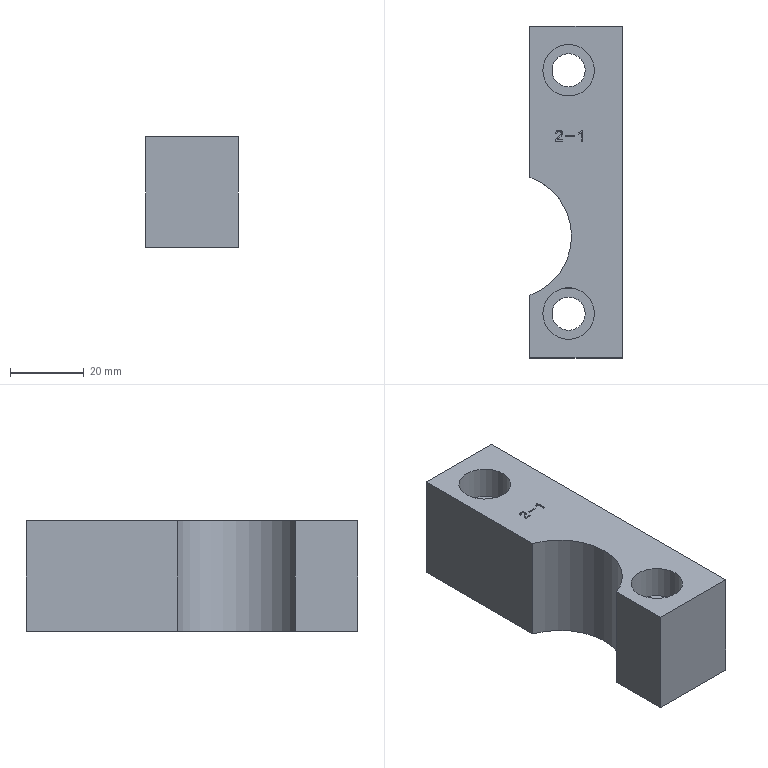Part | STEP file | solid 20 | 1 solid | 34 faces | box 25 x 90 x 30 mm | volume 54142 mm3 | plane 25 | cylinder 5 | other 4 | commonest cylinder face diameters 9 x2 14 x2 34 x1